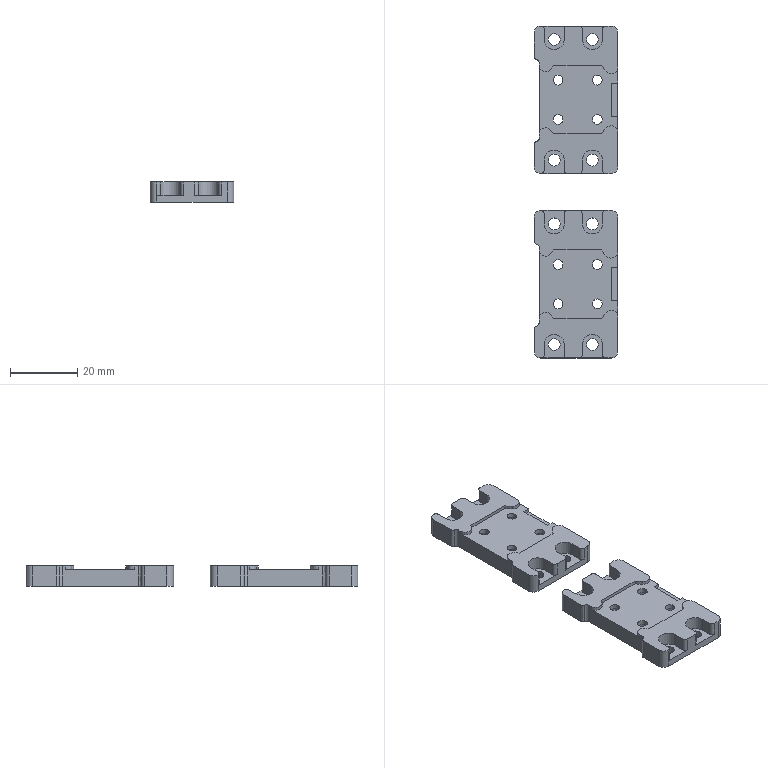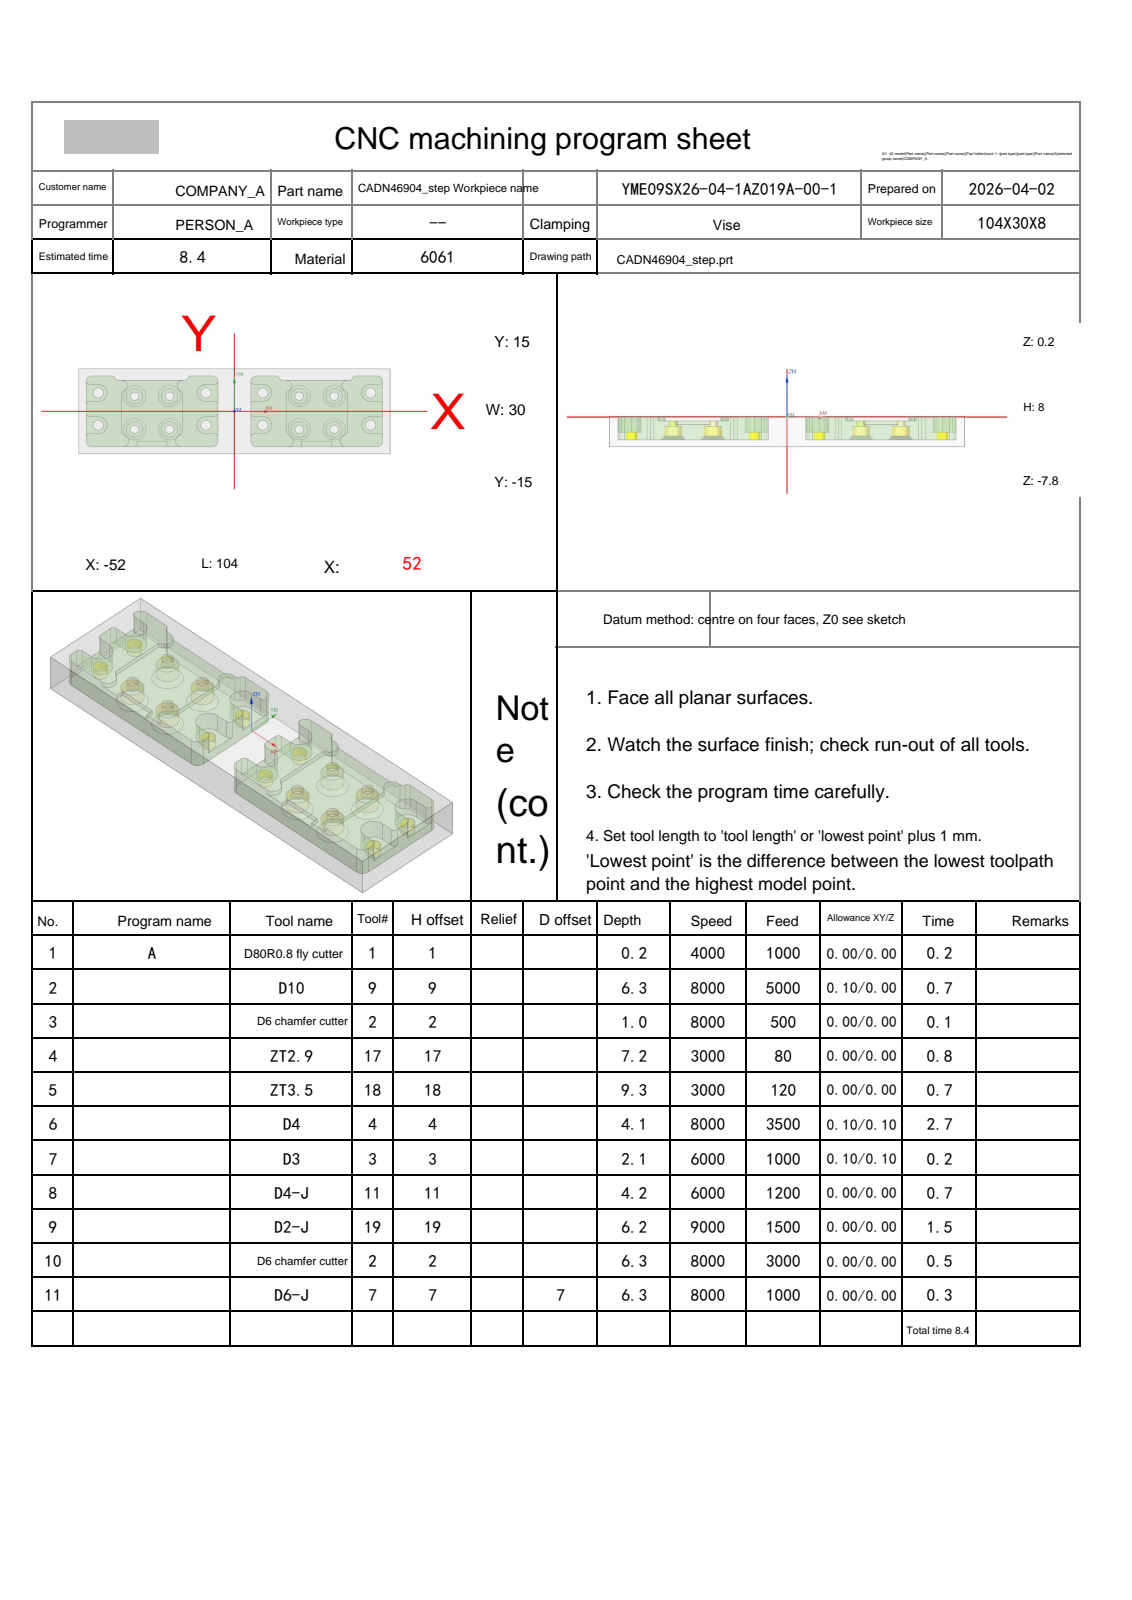NC program | NX | posted by the shop | part box 25 x 99 x 6 mm
Lines 1 to 2900 of 9316, first 1940 of 2898 lines:
%
O0001
(Machine time: 10.55 MIN)
(===Total Tool:10===)
(T1=D80R0.8 fly cutter D=80.  R=0.8  D-  H01 Z=-0.   )
(T9=D10     D=10.  R=0.   D-  H09 Z=-6.1  )
(T2=D6 chamfer cutter   D=6.   R=0.   D-  H02 Z=-6.05 )
(T17=ZT2.9  D=2.9  DR_a=120 D-  H17 Z=-7.   )
(T18=ZT3.5  D=3.5  DR_a=118 D-  H18 Z=-9.05 )
(T4=D4      D=4.   R=0.   D-  H04 Z=-3.9  )
(T3=D3      D=3.   R=0.   D-  H03 Z=-1.9  )
(T11=D4-J   D=4.   R=0.   D11 H11 Z=-4.   )
(T19=D2-J   D=2.   R=0.   D19 H19 Z=-5.95 )
(T7=D6-J    D=6.   R=0.   D7  H07 Z=-6.1  )
G80 G90 G17 G49 G40
G91 G28 Z0
M01
N1 T01 M06
(D80R0.8 fly cutter  D=80. R=0.8 H=01 ce=0.00 di=0.00)
G00 G90 G54 X-94.5 Y0.0 M03 S4000
G43 H01 Z20.
M08
Z2.
G01 Z0.0 F1000.
X-89.5
X89.5
X94.5
Z2.
G00 Z20.
G91 G28 Z0.0
M05
M09
G91 G28 Z0.0
M01
N2 T09 M06
(D10  D=10. R=0. H=09 ce=0.10 di=0.00)
G00 G90 G54 X-27.5 Y-17.6 M03 S8000
G43 H09 Z20.
M08
Z.5
G01 X-47.5 Z.412 F5000.
G02 X-54.6 Y-10.5 Z.363 I0.0 J7.1
G01 Y10.5 Z.271
G02 X-47.5 Y17.6 Z.223 I7.1 J0.0
G01 X-40.936 Z.194
G02 X-36.93 Y16.1 Z.175 I0.0 J-6.1
G01 X-18.57 Z.094
G02 X-14.564 Y17.6 Z.075 I4.006 J-4.6
G01 X-7.5 Z.044
G02 X-.4 Y10.5 Z-.005 I0.0 J-7.1
G01 Y-10.5 Z-.097
G02 X-7.5 Y-17.6 Z-.146 I-7.1 J0.0
G01 X-47.5 Z-.321
G02 X-54.6 Y-10.5 Z-.37 I0.0 J7.1
G01 Y10.5 Z-.462
G02 X-47.5 Y17.6 Z-.511 I7.1 J0.0
G01 X-40.936 Z-.54
G02 X-36.93 Y16.1 Z-.559 I0.0 J-6.1
G01 X-18.57 Z-.639
G02 X-14.564 Y17.6 Z-.658 I4.006 J-4.6
G01 X-7.5 Z-.689
G02 X-.4 Y10.5 Z-.738 I0.0 J-7.1
G01 Y-10.5 Z-.83
G02 X-7.5 Y-17.6 Z-.879 I-7.1 J0.0
G01 X-47.5 Z-1.054
G02 X-54.6 Y-10.5 Z-1.103 I0.0 J7.1
G01 Y10.5 Z-1.195
G02 X-47.5 Y17.6 Z-1.244 I7.1 J0.0
G01 X-40.936 Z-1.273
G02 X-36.93 Y16.1 Z-1.292 I0.0 J-6.1
G01 X-18.57 Z-1.372
G02 X-14.564 Y17.6 Z-1.392 I4.006 J-4.6
G01 X-7.5 Z-1.423
G02 X-.4 Y10.5 Z-1.471 I0.0 J-7.1
G01 Y-10.5 Z-1.563
G02 X-7.5 Y-17.6 Z-1.612 I-7.1 J0.0
G01 X-47.5 Z-1.788
G02 X-54.6 Y-10.5 Z-1.837 I0.0 J7.1
G01 Y10.5 Z-1.929
G02 X-47.5 Y17.6 Z-1.977 I7.1 J0.0
G01 X-40.936 Z-2.006
G02 X-36.93 Y16.1 Z-2.025 I0.0 J-6.1
G01 X-18.57 Z-2.106
G02 X-14.564 Y17.6 Z-2.125 I4.006 J-4.6
G01 X-7.5 Z-2.156
G02 X-.4 Y10.5 Z-2.205 I0.0 J-7.1
G01 Y-10.5 Z-2.297
G02 X-7.5 Y-17.6 Z-2.346 I-7.1 J0.0
G01 X-47.5 Z-2.521
G02 X-54.6 Y-10.5 Z-2.57 I0.0 J7.1
G01 Y10.5 Z-2.662
G02 X-47.5 Y17.6 Z-2.711 I7.1 J0.0
G01 X-40.936 Z-2.74
G02 X-36.93 Y16.1 Z-2.759 I0.0 J-6.1
G01 X-18.57 Z-2.839
G02 X-14.564 Y17.6 Z-2.858 I4.006 J-4.6
G01 X-7.5 Z-2.889
G02 X-.4 Y10.5 Z-2.938 I0.0 J-7.1
G01 Y-10.5 Z-3.03
G02 X-7.5 Y-17.6 Z-3.079 I-7.1 J0.0
G01 X-47.5 Z-3.254
G02 X-54.6 Y-10.5 Z-3.303 I0.0 J7.1
G01 Y10.5 Z-3.395
G02 X-47.5 Y17.6 Z-3.444 I7.1 J0.0
G01 X-40.936 Z-3.473
G02 X-36.93 Y16.1 Z-3.492 I0.0 J-6.1
G01 X-18.57 Z-3.572
G02 X-14.564 Y17.6 Z-3.592 I4.006 J-4.6
G01 X-7.5 Z-3.623
G02 X-.4 Y10.5 Z-3.671 I0.0 J-7.1
G01 Y-10.5 Z-3.763
G02 X-7.5 Y-17.6 Z-3.812 I-7.1 J0.0
G01 X-47.5 Z-3.988
G02 X-54.6 Y-10.5 Z-4.037 I0.0 J7.1
G01 Y10.5 Z-4.129
G02 X-47.5 Y17.6 Z-4.177 I7.1 J0.0
G01 X-40.936 Z-4.206
G02 X-36.93 Y16.1 Z-4.225 I0.0 J-6.1
G01 X-18.57 Z-4.306
G02 X-14.564 Y17.6 Z-4.325 I4.006 J-4.6
G01 X-7.5 Z-4.356
G02 X-.4 Y10.5 Z-4.405 I0.0 J-7.1
G01 Y-10.5 Z-4.497
G02 X-7.5 Y-17.6 Z-4.546 I-7.1 J0.0
G01 X-47.5 Z-4.721
G02 X-54.6 Y-10.5 Z-4.77 I0.0 J7.1
G01 Y10.5 Z-4.862
G02 X-47.5 Y17.6 Z-4.911 I7.1 J0.0
G01 X-40.936 Z-4.94
G02 X-36.93 Y16.1 Z-4.959 I0.0 J-6.1
G01 X-18.57 Z-5.039
G02 X-14.564 Y17.6 Z-5.058 I4.006 J-4.6
G01 X-7.5 Z-5.089
G02 X-.4 Y10.5 Z-5.138 I0.0 J-7.1
G01 Y-10.5 Z-5.23
G02 X-7.5 Y-17.6 Z-5.279 I-7.1 J0.0
G01 X-47.5 Z-5.454
G02 X-54.6 Y-10.5 Z-5.503 I0.0 J7.1
G01 Y10.5 Z-5.595
G02 X-47.5 Y17.6 Z-5.644 I7.1 J0.0
G01 X-40.936 Z-5.673
G02 X-36.93 Y16.1 Z-5.692 I0.0 J-6.1
G01 X-18.57 Z-5.772
G02 X-14.564 Y17.6 Z-5.792 I4.006 J-4.6
G01 X-7.5 Z-5.823
G02 X-.4 Y10.5 Z-5.871 I0.0 J-7.1
G01 Y-10.5 Z-5.963
G02 X-7.5 Y-17.6 Z-6.012 I-7.1 J0.0
G01 X-27.5 Z-6.1
X-47.5
G02 X-54.6 Y-10.5 I0.0 J7.1
G01 Y10.5
G02 X-47.5 Y17.6 I7.1 J0.0
G01 X-40.936
G02 X-36.93 Y16.1 I0.0 J-6.1
G01 X-18.57
G02 X-14.564 Y17.6 I4.006 J-4.6
G01 X-7.5
G02 X-.4 Y10.5 I0.0 J-7.1
G01 Y-10.5
G02 X-7.5 Y-17.6 I-7.1 J0.0
G01 X-27.5
X-28.
Z-5.1
G00 Z20.
X27.5
Z.5
G01 X7.5 Z.412
G02 X.4 Y-10.5 Z.363 I0.0 J7.1
G01 Y10.5 Z.271
G02 X7.5 Y17.6 Z.223 I7.1 J0.0
G01 X14.064 Z.194
G02 X18.07 Y16.1 Z.175 I0.0 J-6.1
G01 X36.43 Z.094
G02 X40.436 Y17.6 Z.075 I4.006 J-4.6
G01 X47.5 Z.044
G02 X54.6 Y10.5 Z-.005 I0.0 J-7.1
G01 Y-10.5 Z-.097
G02 X47.5 Y-17.6 Z-.146 I-7.1 J0.0
G01 X7.5 Z-.321
G02 X.4 Y-10.5 Z-.37 I0.0 J7.1
G01 Y10.5 Z-.462
G02 X7.5 Y17.6 Z-.511 I7.1 J0.0
G01 X14.064 Z-.54
G02 X18.07 Y16.1 Z-.559 I0.0 J-6.1
G01 X36.43 Z-.639
G02 X40.436 Y17.6 Z-.658 I4.006 J-4.6
G01 X47.5 Z-.689
G02 X54.6 Y10.5 Z-.738 I0.0 J-7.1
G01 Y-10.5 Z-.83
G02 X47.5 Y-17.6 Z-.879 I-7.1 J0.0
G01 X7.5 Z-1.054
G02 X.4 Y-10.5 Z-1.103 I0.0 J7.1
G01 Y10.5 Z-1.195
G02 X7.5 Y17.6 Z-1.244 I7.1 J0.0
G01 X14.064 Z-1.273
G02 X18.07 Y16.1 Z-1.292 I0.0 J-6.1
G01 X36.43 Z-1.372
G02 X40.436 Y17.6 Z-1.392 I4.006 J-4.6
G01 X47.5 Z-1.423
G02 X54.6 Y10.5 Z-1.471 I0.0 J-7.1
G01 Y-10.5 Z-1.563
G02 X47.5 Y-17.6 Z-1.612 I-7.1 J0.0
G01 X7.5 Z-1.788
G02 X.4 Y-10.5 Z-1.837 I0.0 J7.1
G01 Y10.5 Z-1.929
G02 X7.5 Y17.6 Z-1.977 I7.1 J0.0
G01 X14.064 Z-2.006
G02 X18.07 Y16.1 Z-2.025 I0.0 J-6.1
G01 X36.43 Z-2.106
G02 X40.436 Y17.6 Z-2.125 I4.006 J-4.6
G01 X47.5 Z-2.156
G02 X54.6 Y10.5 Z-2.205 I0.0 J-7.1
G01 Y-10.5 Z-2.297
G02 X47.5 Y-17.6 Z-2.346 I-7.1 J0.0
G01 X7.5 Z-2.521
G02 X.4 Y-10.5 Z-2.57 I0.0 J7.1
G01 Y10.5 Z-2.662
G02 X7.5 Y17.6 Z-2.711 I7.1 J0.0
G01 X14.064 Z-2.74
G02 X18.07 Y16.1 Z-2.759 I0.0 J-6.1
G01 X36.43 Z-2.839
G02 X40.436 Y17.6 Z-2.858 I4.006 J-4.6
G01 X47.5 Z-2.889
G02 X54.6 Y10.5 Z-2.938 I0.0 J-7.1
G01 Y-10.5 Z-3.03
G02 X47.5 Y-17.6 Z-3.079 I-7.1 J0.0
G01 X7.5 Z-3.254
G02 X.4 Y-10.5 Z-3.303 I0.0 J7.1
G01 Y10.5 Z-3.395
G02 X7.5 Y17.6 Z-3.444 I7.1 J0.0
G01 X14.064 Z-3.473
G02 X18.07 Y16.1 Z-3.492 I0.0 J-6.1
G01 X36.43 Z-3.572
G02 X40.436 Y17.6 Z-3.592 I4.006 J-4.6
G01 X47.5 Z-3.623
G02 X54.6 Y10.5 Z-3.671 I0.0 J-7.1
G01 Y-10.5 Z-3.763
G02 X47.5 Y-17.6 Z-3.812 I-7.1 J0.0
G01 X7.5 Z-3.988
G02 X.4 Y-10.5 Z-4.037 I0.0 J7.1
G01 Y10.5 Z-4.129
G02 X7.5 Y17.6 Z-4.177 I7.1 J0.0
G01 X14.064 Z-4.206
G02 X18.07 Y16.1 Z-4.225 I0.0 J-6.1
G01 X36.43 Z-4.306
G02 X40.436 Y17.6 Z-4.325 I4.006 J-4.6
G01 X47.5 Z-4.356
G02 X54.6 Y10.5 Z-4.405 I0.0 J-7.1
G01 Y-10.5 Z-4.497
G02 X47.5 Y-17.6 Z-4.546 I-7.1 J0.0
G01 X7.5 Z-4.721
G02 X.4 Y-10.5 Z-4.77 I0.0 J7.1
G01 Y10.5 Z-4.862
G02 X7.5 Y17.6 Z-4.911 I7.1 J0.0
G01 X14.064 Z-4.94
G02 X18.07 Y16.1 Z-4.959 I0.0 J-6.1
G01 X36.43 Z-5.039
G02 X40.436 Y17.6 Z-5.058 I4.006 J-4.6
G01 X47.5 Z-5.089
G02 X54.6 Y10.5 Z-5.138 I0.0 J-7.1
G01 Y-10.5 Z-5.23
G02 X47.5 Y-17.6 Z-5.279 I-7.1 J0.0
G01 X7.5 Z-5.454
G02 X.4 Y-10.5 Z-5.503 I0.0 J7.1
G01 Y10.5 Z-5.595
G02 X7.5 Y17.6 Z-5.644 I7.1 J0.0
G01 X14.064 Z-5.673
G02 X18.07 Y16.1 Z-5.692 I0.0 J-6.1
G01 X36.43 Z-5.772
G02 X40.436 Y17.6 Z-5.792 I4.006 J-4.6
G01 X47.5 Z-5.823
G02 X54.6 Y10.5 Z-5.871 I0.0 J-7.1
G01 Y-10.5 Z-5.963
G02 X47.5 Y-17.6 Z-6.012 I-7.1 J0.0
G01 X32.5 Z-6.078
X27.5 Z-6.1
X7.5
G02 X.4 Y-10.5 I0.0 J7.1
G01 Y10.5
G02 X7.5 Y17.6 I7.1 J0.0
G01 X14.064
G02 X18.07 Y16.1 I0.0 J-6.1
G01 X36.43
G02 X40.436 Y17.6 I4.006 J-4.6
G01 X47.5
G02 X54.6 Y10.5 I0.0 J-7.1
G01 Y-10.5
G02 X47.5 Y-17.6 I-7.1 J0.0
G01 X32.5
X27.5
X27.
Z-5.1
G00 Z20.
G91 G28 Z0.0
M05
M09
G91 G28 Z0.0
M01
N3 T02 M06
(D6 chamfer cutter  D=6. R=0. H=02 ce=0.00 di=0.00)
G00 G90 G54 X45.5 Y6.5 M03 S8000
G43 H02 Z20.
M08
G98 G81 X45.5 Y6.5 Z-.8 R1. F500.
Y-4.881
X33.338 Y-6.33
X33.329 Y5.329
X21.662
X21.671 Y-6.338
X9.5 Y-4.881
Y6.5
X-9.5
Y-4.881
X-21.662 Y-6.33
X-21.671 Y5.329
X-33.338
X-33.329 Y-6.338
X-45.5 Y-4.881
Y6.5
G80
G00 Z20.
G91 G28 Z0.0
M05
M09
G91 G28 Z0.0
M01
N4 T17 M06
(ZT2.9 D=2.9 DR_a=120 H=17)
G00 G90 G54 X-33.338 Y5.329 M03 S3000
G43 H17 Z20.
M08
G98 G83 X-33.338 Y5.329 Z-7. R1. F80. Q2.5
X-33.329 Y-6.338
X-21.662 Y-6.33
X-21.671 Y5.329
X21.662
X33.329
X33.338 Y-6.33
X21.671 Y-6.338
G80
G00 Z20.
G91 G28 Z0.0
M05
M09
G91 G28 Z0.0
M01
N5 T18 M06
(ZT3.5 D=3.5 DR_a=118 H=18)
G00 G90 G54 X-45.5 Y-4.881 M03 S3000
G43 H18 Z20.
M08
G98 G83 X-45.5 Y-4.881 Z-9.052 R1. F120. Q3.
Y6.5
X-9.5
Y-4.881
X9.5
Y6.5
X45.5
Y-4.881
G80
G00 Z20.
G91 G28 Z0.0
M05
M09
G91 G28 Z0.0
M01
N6 T04 M06
(D4  D=4. R=0. H=04 ce=0.10 di=0.10)
G00 G90 G54 X-27.5 Y-15.5 M03 S8000
G43 H04 Z20.
M08
Z.275
G01 Z-.225 F3500.
Y-10.9
X-32.1
Y-12.9
X-33.974
G03 X-33.198 Y-10.5 I-3.324 J2.4
X-34.426 Y-7.574 I-4.1 J0.0
X-35.6 Y-6.543 I-9.876 J-10.064
G01 Y5.543
G03 X-35.2 Y5.869 I-8.702 J11.094
X-33.747 Y9. I-2.647 J3.131
X-34.523 Y11.4 I-4.1 J0.0
G01 X-20.477
G03 X-21.253 Y9. I3.324 J-2.4
X-19.8 Y5.869 I4.1 J0.0
X-19.4 Y5.543 I9.102 J10.769
G01 Y-6.543
G03 X-20.574 Y-7.574 I8.702 J-11.094
X-21.802 Y-10.5 I2.872 J-2.926
X-21.026 Y-12.9 I4.1 J0.0
G01 X-22.9
Y-10.9
X-27.5
Y-8.1
X-30.829
G03 X-32.465 Y-5.575 I-6.469 J-2.4
X-32.8 Y-5.255 I-11.837 J-12.062
G01 Y4.295
G03 X-30.958 Y8.6 I-5.047 J4.705
G01 X-24.042
G03 X-22.2 Y4.295 I6.888 J.4
G01 Y-5.255
G03 X-22.535 Y-5.575 I11.502 J-12.382
X-24.171 Y-8.1 I4.833 J-4.925
G01 X-27.5
Y-5.3
X-29.11
G03 X-30. Y-4.11 I-8.188 J-5.2
G01 Y3.298
G03 X-28.69 Y5.8 I-7.847 J5.702
G01 X-26.31
G03 X-25. Y3.298 I9.157 J3.2
G01 Y-4.11
G03 X-25.89 Y-5.3 I7.298 J-6.39
G01 X-27.5
Y-3.5
X-28.174
X-28.2 Y-3.466
Y2.74
G03 X-27.5 Y3.981 I-9.647 J6.26
X-26.8 Y2.74 I10.347 J5.019
G01 Y-3.466
X-26.826 Y-3.5
X-27.5
X-28.
Z.275
G00 Z.5
X-27.5 Y-15.5
Z.05
G01 Z-.45
Y-10.9
X-32.1
Y-12.9
X-33.974
G03 X-33.198 Y-10.5 I-3.324 J2.4
X-34.426 Y-7.574 I-4.1 J0.0
X-35.6 Y-6.543 I-9.876 J-10.064
G01 Y5.543
G03 X-35.2 Y5.869 I-8.702 J11.094
X-33.747 Y9. I-2.647 J3.131
X-34.523 Y11.4 I-4.1 J0.0
G01 X-20.477
G03 X-21.253 Y9. I3.324 J-2.4
X-19.8 Y5.869 I4.1 J0.0
X-19.4 Y5.543 I9.102 J10.769
G01 Y-6.543
G03 X-20.574 Y-7.574 I8.702 J-11.094
X-21.802 Y-10.5 I2.872 J-2.926
X-21.026 Y-12.9 I4.1 J0.0
G01 X-22.9
Y-10.9
X-27.5
Y-8.1
X-30.829
G03 X-32.465 Y-5.575 I-6.469 J-2.4
X-32.8 Y-5.255 I-11.837 J-12.062
G01 Y4.295
G03 X-30.958 Y8.6 I-5.047 J4.705
G01 X-24.042
G03 X-22.2 Y4.295 I6.888 J.4
G01 Y-5.255
G03 X-22.535 Y-5.575 I11.502 J-12.382
X-24.171 Y-8.1 I4.833 J-4.925
G01 X-27.5
Y-5.3
X-29.11
G03 X-30. Y-4.11 I-8.188 J-5.2
G01 Y3.298
G03 X-28.69 Y5.8 I-7.847 J5.702
G01 X-26.31
G03 X-25. Y3.298 I9.157 J3.2
G01 Y-4.11
G03 X-25.89 Y-5.3 I7.298 J-6.39
G01 X-27.5
Y-3.5
X-28.174
X-28.2 Y-3.466
Y2.74
G03 X-27.5 Y3.981 I-9.647 J6.26
X-26.8 Y2.74 I10.347 J5.019
G01 Y-3.466
X-26.826 Y-3.5
X-27.5
X-28.
Z.05
G00 Z.275
X-27.5 Y-15.5
Z-.175
G01 Z-.675
Y-10.9
X-32.1
Y-12.9
X-33.974
G03 X-33.198 Y-10.5 I-3.324 J2.4
X-34.426 Y-7.574 I-4.1 J0.0
X-35.6 Y-6.543 I-9.876 J-10.064
G01 Y5.543
G03 X-35.2 Y5.869 I-8.702 J11.094
X-33.747 Y9. I-2.647 J3.131
X-34.523 Y11.4 I-4.1 J0.0
G01 X-20.477
G03 X-21.253 Y9. I3.324 J-2.4
X-19.8 Y5.869 I4.1 J0.0
X-19.4 Y5.543 I9.102 J10.769
G01 Y-6.543
G03 X-20.574 Y-7.574 I8.702 J-11.094
X-21.802 Y-10.5 I2.872 J-2.926
X-21.026 Y-12.9 I4.1 J0.0
G01 X-22.9
Y-10.9
X-27.5
Y-8.1
X-30.829
G03 X-32.465 Y-5.575 I-6.469 J-2.4
X-32.8 Y-5.255 I-11.837 J-12.062
G01 Y4.295
G03 X-30.958 Y8.6 I-5.047 J4.705
G01 X-24.042
G03 X-22.2 Y4.295 I6.888 J.4
G01 Y-5.255
G03 X-22.535 Y-5.575 I11.502 J-12.382
X-24.171 Y-8.1 I4.833 J-4.925
G01 X-27.5
Y-5.3
X-29.11
G03 X-30. Y-4.11 I-8.188 J-5.2
G01 Y3.298
G03 X-28.69 Y5.8 I-7.847 J5.702
G01 X-26.31
G03 X-25. Y3.298 I9.157 J3.2
G01 Y-4.11
G03 X-25.89 Y-5.3 I7.298 J-6.39
G01 X-27.5
Y-3.5
X-28.174
X-28.2 Y-3.466
Y2.74
G03 X-27.5 Y3.981 I-9.647 J6.26
X-26.8 Y2.74 I10.347 J5.019
G01 Y-3.466
X-26.826 Y-3.5
X-27.5
X-28.
Z-.175
G00 Z.05
X-27.5 Y-15.5
Z-.4
G01 Z-.9
Y-10.9
X-32.1
Y-12.9
X-33.974
G03 X-33.198 Y-10.5 I-3.324 J2.4
X-34.426 Y-7.574 I-4.1 J0.0
X-35.6 Y-6.543 I-9.876 J-10.064
G01 Y5.543
G03 X-35.2 Y5.869 I-8.702 J11.094
X-33.747 Y9. I-2.647 J3.131
X-34.523 Y11.4 I-4.1 J0.0
G01 X-20.477
G03 X-21.253 Y9. I3.324 J-2.4
X-19.8 Y5.869 I4.1 J0.0
X-19.4 Y5.543 I9.102 J10.769
G01 Y-6.543
G03 X-20.574 Y-7.574 I8.702 J-11.094
X-21.802 Y-10.5 I2.872 J-2.926
X-21.026 Y-12.9 I4.1 J0.0
G01 X-22.9
Y-10.9
X-27.5
Y-8.1
X-30.829
G03 X-32.465 Y-5.575 I-6.469 J-2.4
X-32.8 Y-5.255 I-11.837 J-12.062
G01 Y4.295
G03 X-30.958 Y8.6 I-5.047 J4.705
G01 X-24.042
G03 X-22.2 Y4.295 I6.888 J.4
G01 Y-5.255
G03 X-22.535 Y-5.575 I11.502 J-12.382
X-24.171 Y-8.1 I4.833 J-4.925
G01 X-27.5
Y-5.3
X-29.11
G03 X-30. Y-4.11 I-8.188 J-5.2
G01 Y3.298
G03 X-28.69 Y5.8 I-7.847 J5.702
G01 X-26.31
G03 X-25. Y3.298 I9.157 J3.2
G01 Y-4.11
G03 X-25.89 Y-5.3 I7.298 J-6.39
G01 X-27.5
Y-3.5
X-28.174
X-28.2 Y-3.466
Y2.74
G03 X-27.5 Y3.981 I-9.647 J6.26
X-26.8 Y2.74 I10.347 J5.019
G01 Y-3.466
X-26.826 Y-3.5
X-27.5
X-28.
Z-.4
G00 Z20.
X27.5 Y-15.5
Z.275
G01 Z-.225
Y-10.9
X22.9
Y-12.9
X21.026
G03 X21.802 Y-10.5 I-3.324 J2.4
X20.574 Y-7.574 I-4.1 J0.0
X19.4 Y-6.543 I-9.876 J-10.064
G01 Y5.543
G03 X19.8 Y5.869 I-8.702 J11.094
X21.253 Y9. I-2.647 J3.131
X20.477 Y11.4 I-4.1 J0.0
G01 X34.523
G03 X33.747 Y9. I3.324 J-2.4
X35.2 Y5.869 I4.1 J0.0
X35.6 Y5.543 I9.102 J10.769
G01 Y-6.543
G03 X34.426 Y-7.574 I8.702 J-11.094
X33.198 Y-10.5 I2.872 J-2.926
X33.974 Y-12.9 I4.1 J0.0
G01 X32.1
Y-10.9
X27.5
Y-8.1
X24.171
G03 X22.535 Y-5.575 I-6.469 J-2.4
X22.2 Y-5.255 I-11.837 J-12.062
G01 Y4.295
G03 X24.042 Y8.6 I-5.047 J4.705
G01 X30.958
G03 X32.8 Y4.295 I6.888 J.4
G01 Y-5.255
G03 X32.465 Y-5.575 I11.502 J-12.382
X30.829 Y-8.1 I4.833 J-4.925
G01 X27.5
Y-5.3
X25.89
G03 X25. Y-4.11 I-8.188 J-5.2
G01 Y3.298
G03 X26.31 Y5.8 I-7.847 J5.702
G01 X28.69
G03 X30. Y3.298 I9.157 J3.2
G01 Y-4.11
G03 X29.11 Y-5.3 I7.298 J-6.39
G01 X27.5
Y-3.5
X26.826
X26.8 Y-3.466
Y2.74
G03 X27.5 Y3.981 I-9.647 J6.26
X28.2 Y2.74 I10.347 J5.019
G01 Y-3.466
X28.174 Y-3.5
X27.5
X27.
Z.275
G00 Z.5
X27.5 Y-15.5
Z.05
G01 Z-.45
Y-10.9
X22.9
Y-12.9
X21.026
G03 X21.802 Y-10.5 I-3.324 J2.4
X20.574 Y-7.574 I-4.1 J0.0
X19.4 Y-6.543 I-9.876 J-10.064
G01 Y5.543
G03 X19.8 Y5.869 I-8.702 J11.094
X21.253 Y9. I-2.647 J3.131
X20.477 Y11.4 I-4.1 J0.0
G01 X34.523
G03 X33.747 Y9. I3.324 J-2.4
X35.2 Y5.869 I4.1 J0.0
X35.6 Y5.543 I9.102 J10.769
G01 Y-6.543
G03 X34.426 Y-7.574 I8.702 J-11.094
X33.198 Y-10.5 I2.872 J-2.926
X33.974 Y-12.9 I4.1 J0.0
G01 X32.1
Y-10.9
X27.5
Y-8.1
X24.171
G03 X22.535 Y-5.575 I-6.469 J-2.4
X22.2 Y-5.255 I-11.837 J-12.062
G01 Y4.295
G03 X24.042 Y8.6 I-5.047 J4.705
G01 X30.958
G03 X32.8 Y4.295 I6.888 J.4
G01 Y-5.255
G03 X32.465 Y-5.575 I11.502 J-12.382
X30.829 Y-8.1 I4.833 J-4.925
G01 X27.5
Y-5.3
X25.89
G03 X25. Y-4.11 I-8.188 J-5.2
G01 Y3.298
G03 X26.31 Y5.8 I-7.847 J5.702
G01 X28.69
G03 X30. Y3.298 I9.157 J3.2
G01 Y-4.11
G03 X29.11 Y-5.3 I7.298 J-6.39
G01 X27.5
Y-3.5
X26.826
X26.8 Y-3.466
Y2.74
G03 X27.5 Y3.981 I-9.647 J6.26
X28.2 Y2.74 I10.347 J5.019
G01 Y-3.466
X28.174 Y-3.5
X27.5
X27.
Z.05
G00 Z.275
X27.5 Y-15.5
Z-.175
G01 Z-.675
Y-10.9
X22.9
Y-12.9
X21.026
G03 X21.802 Y-10.5 I-3.324 J2.4
X20.574 Y-7.574 I-4.1 J0.0
X19.4 Y-6.543 I-9.876 J-10.064
G01 Y5.543
G03 X19.8 Y5.869 I-8.702 J11.094
X21.253 Y9. I-2.647 J3.131
X20.477 Y11.4 I-4.1 J0.0
G01 X34.523
G03 X33.747 Y9. I3.324 J-2.4
X35.2 Y5.869 I4.1 J0.0
X35.6 Y5.543 I9.102 J10.769
G01 Y-6.543
G03 X34.426 Y-7.574 I8.702 J-11.094
X33.198 Y-10.5 I2.872 J-2.926
X33.974 Y-12.9 I4.1 J0.0
G01 X32.1
Y-10.9
X27.5
Y-8.1
X24.171
G03 X22.535 Y-5.575 I-6.469 J-2.4
X22.2 Y-5.255 I-11.837 J-12.062
G01 Y4.295
G03 X24.042 Y8.6 I-5.047 J4.705
G01 X30.958
G03 X32.8 Y4.295 I6.888 J.4
G01 Y-5.255
G03 X32.465 Y-5.575 I11.502 J-12.382
X30.829 Y-8.1 I4.833 J-4.925
G01 X27.5
Y-5.3
X25.89
G03 X25. Y-4.11 I-8.188 J-5.2
G01 Y3.298
G03 X26.31 Y5.8 I-7.847 J5.702
G01 X28.69
G03 X30. Y3.298 I9.157 J3.2
G01 Y-4.11
G03 X29.11 Y-5.3 I7.298 J-6.39
G01 X27.5
Y-3.5
X26.826
X26.8 Y-3.466
Y2.74
G03 X27.5 Y3.981 I-9.647 J6.26
X28.2 Y2.74 I10.347 J5.019
G01 Y-3.466
X28.174 Y-3.5
X27.5
X27.
Z-.175
G00 Z.05
X27.5 Y-15.5
Z-.4
G01 Z-.9
Y-10.9
X22.9
Y-12.9
X21.026
G03 X21.802 Y-10.5 I-3.324 J2.4
X20.574 Y-7.574 I-4.1 J0.0
X19.4 Y-6.543 I-9.876 J-10.064
G01 Y5.543
G03 X19.8 Y5.869 I-8.702 J11.094
X21.253 Y9. I-2.647 J3.131
X20.477 Y11.4 I-4.1 J0.0
G01 X34.523
G03 X33.747 Y9. I3.324 J-2.4
X35.2 Y5.869 I4.1 J0.0
X35.6 Y5.543 I9.102 J10.769
G01 Y-6.543
G03 X34.426 Y-7.574 I8.702 J-11.094
X33.198 Y-10.5 I2.872 J-2.926
X33.974 Y-12.9 I4.1 J0.0
G01 X32.1
Y-10.9
X27.5
Y-8.1
X24.171
G03 X22.535 Y-5.575 I-6.469 J-2.4
X22.2 Y-5.255 I-11.837 J-12.062
G01 Y4.295
G03 X24.042 Y8.6 I-5.047 J4.705
G01 X30.958
G03 X32.8 Y4.295 I6.888 J.4
G01 Y-5.255
G03 X32.465 Y-5.575 I11.502 J-12.382
X30.829 Y-8.1 I4.833 J-4.925
G01 X27.5
Y-5.3
X25.89
G03 X25. Y-4.11 I-8.188 J-5.2
G01 Y3.298
G03 X26.31 Y5.8 I-7.847 J5.702
G01 X28.69
G03 X30. Y3.298 I9.157 J3.2
G01 Y-4.11
G03 X29.11 Y-5.3 I7.298 J-6.39
G01 X27.5
Y-3.5
X26.826
X26.8 Y-3.466
Y2.74
G03 X27.5 Y3.981 I-9.647 J6.26
X28.2 Y2.74 I10.347 J5.019
G01 Y-3.466
X28.174 Y-3.5
X27.5
X27.
Z-.4
G00 Z20.
G00 G90 X-54.5 Y-4.881 M03 S8000
Z20.
Z.256
G01 Z-.244 F1200.
X-49.9
Y-6.115
G02 X-48.5 Y-5.781 I1.4 J-2.766
G01 X-45.5
G03 X-44.6 Y-4.881 I0.0 J.9
X-45.5 Y-3.981 I-.9 J0.0
G01 X-48.5
G02 X-49.9 Y-3.646 I0.0 J3.1
G01 Y-4.881
Y-5.381
Z.256
G00 Z.5
X-54.5 Y-4.881
Z.013
G01 Z-.488
X-49.9
Y-6.115
G02 X-48.5 Y-5.781 I1.4 J-2.766
G01 X-45.5
G03 X-44.6 Y-4.881 I0.0 J.9
X-45.5 Y-3.981 I-.9 J0.0
G01 X-48.5
G02 X-49.9 Y-3.646 I0.0 J3.1
G01 Y-4.881
Y-5.381
Z.013
G00 Z.256
X-54.5 Y-4.881
Z-.231
G01 Z-.731
X-49.9
Y-6.115
G02 X-48.5 Y-5.781 I1.4 J-2.766
G01 X-45.5
G03 X-44.6 Y-4.881 I0.0 J.9
X-45.5 Y-3.981 I-.9 J0.0
G01 X-48.5
G02 X-49.9 Y-3.646 I0.0 J3.1
G01 Y-4.881
Y-5.381
Z-.231
G00 Z.013
X-54.5 Y-4.881
Z-.475
G01 Z-.975
X-49.9
Y-6.115
G02 X-48.5 Y-5.781 I1.4 J-2.766
G01 X-45.5
G03 X-44.6 Y-4.881 I0.0 J.9
X-45.5 Y-3.981 I-.9 J0.0
G01 X-48.5
G02 X-49.9 Y-3.646 I0.0 J3.1
G01 Y-4.881
Y-5.381
Z-.475
G00 Z-.231
X-54.5 Y-4.881
Z-.719
G01 Z-1.219
X-49.9
Y-6.115
G02 X-48.5 Y-5.781 I1.4 J-2.766
G01 X-45.5
G03 X-44.6 Y-4.881 I0.0 J.9
X-45.5 Y-3.981 I-.9 J0.0
G01 X-48.5
G02 X-49.9 Y-3.646 I0.0 J3.1
G01 Y-4.881
Y-5.381
Z-.719
G00 Z-.475
X-54.5 Y-4.881
Z-.963
G01 Z-1.463
X-49.9
Y-6.115
G02 X-48.5 Y-5.781 I1.4 J-2.766
G01 X-45.5
G03 X-44.6 Y-4.881 I0.0 J.9
X-45.5 Y-3.981 I-.9 J0.0
G01 X-48.5
G02 X-49.9 Y-3.646 I0.0 J3.1
G01 Y-4.881
Y-5.381
Z-.963
G00 Z-.719
X-54.5 Y-4.881
Z-1.206
G01 Z-1.706
X-49.9
Y-6.115
G02 X-48.5 Y-5.781 I1.4 J-2.766
G01 X-45.5
G03 X-44.6 Y-4.881 I0.0 J.9
X-45.5 Y-3.981 I-.9 J0.0
G01 X-48.5
G02 X-49.9 Y-3.646 I0.0 J3.1
G01 Y-4.881
Y-5.381
Z-1.206
G00 Z-.963
X-54.5 Y-4.881
Z-1.45
G01 Z-1.95
X-49.9
Y-6.115
G02 X-48.5 Y-5.781 I1.4 J-2.766
G01 X-45.5
G03 X-44.6 Y-4.881 I0.0 J.9
X-45.5 Y-3.981 I-.9 J0.0
G01 X-48.5
G02 X-49.9 Y-3.646 I0.0 J3.1
G01 Y-4.881
Y-5.381
Z-1.45
G00 Z-1.206
X-54.5 Y-4.881
Z-1.694
G01 Z-2.194
X-49.9
Y-6.115
G02 X-48.5 Y-5.781 I1.4 J-2.766
G01 X-45.5
G03 X-44.6 Y-4.881 I0.0 J.9
X-45.5 Y-3.981 I-.9 J0.0
G01 X-48.5
G02 X-49.9 Y-3.646 I0.0 J3.1
G01 Y-4.881
Y-5.381
Z-1.694
G00 Z-1.45
X-54.5 Y-4.881
Z-1.938
G01 Z-2.438
X-49.9
Y-6.115
G02 X-48.5 Y-5.781 I1.4 J-2.766
G01 X-45.5
G03 X-44.6 Y-4.881 I0.0 J.9
X-45.5 Y-3.981 I-.9 J0.0
G01 X-48.5
G02 X-49.9 Y-3.646 I0.0 J3.1
G01 Y-4.881
Y-5.381
Z-1.938
G00 Z-1.694
X-54.5 Y-4.881
Z-2.181
G01 Z-2.681
X-49.9
Y-6.115
G02 X-48.5 Y-5.781 I1.4 J-2.766
G01 X-45.5
G03 X-44.6 Y-4.881 I0.0 J.9
X-45.5 Y-3.981 I-.9 J0.0
G01 X-48.5
G02 X-49.9 Y-3.646 I0.0 J3.1
G01 Y-4.881
Y-5.381
Z-2.181
G00 Z-1.938
X-54.5 Y-4.881
Z-2.425
G01 Z-2.925
X-49.9
Y-6.115
G02 X-48.5 Y-5.781 I1.4 J-2.766
G01 X-45.5
G03 X-44.6 Y-4.881 I0.0 J.9
X-45.5 Y-3.981 I-.9 J0.0
G01 X-48.5
G02 X-49.9 Y-3.646 I0.0 J3.1
G01 Y-4.881
Y-5.381
Z-2.425
G00 Z-2.181
X-54.5 Y-4.881
Z-2.669
G01 Z-3.169
X-49.9
Y-6.115
G02 X-48.5 Y-5.781 I1.4 J-2.766
G01 X-45.5
G03 X-44.6 Y-4.881 I0.0 J.9
X-45.5 Y-3.981 I-.9 J0.0
G01 X-48.5
G02 X-49.9 Y-3.646 I0.0 J3.1
G01 Y-4.881
Y-5.381
Z-2.669
G00 Z-2.425
X-54.5 Y-4.881
Z-2.913
G01 Z-3.413
X-49.9
Y-6.115
G02 X-48.5 Y-5.781 I1.4 J-2.766
G01 X-45.5
G03 X-44.6 Y-4.881 I0.0 J.9
X-45.5 Y-3.981 I-.9 J0.0
G01 X-48.5
G02 X-49.9 Y-3.646 I0.0 J3.1
G01 Y-4.881
Y-5.381
Z-2.913
G00 Z-2.669
X-54.5 Y-4.881
Z-3.156
G01 Z-3.656
X-49.9
Y-6.115
G02 X-48.5 Y-5.781 I1.4 J-2.766
G01 X-45.5
G03 X-44.6 Y-4.881 I0.0 J.9
X-45.5 Y-3.981 I-.9 J0.0
G01 X-48.5
G02 X-49.9 Y-3.646 I0.0 J3.1
G01 Y-4.881
Y-5.381
Z-3.156
G00 Z-2.913
X-54.5 Y-4.881
Z-3.4
G01 Z-3.9
X-49.9
Y-6.115
G02 X-48.5 Y-5.781 I1.4 J-2.766
G01 X-45.5
G03 X-44.6 Y-4.881 I0.0 J.9
X-45.5 Y-3.981 I-.9 J0.0
G01 X-48.5
G02 X-49.9 Y-3.646 I0.0 J3.1
G01 Y-4.881
Y-5.381
Z-3.4
G00 Z20.
X-54.5 Y6.5
Z.256
G01 Z-.244
X-49.9
Y5.266
G02 X-48.5 Y5.6 I1.4 J-2.766
G01 X-45.5
G03 X-44.6 Y6.5 I0.0 J.9
X-45.5 Y7.4 I-.9 J0.0
G01 X-48.5
G02 X-49.9 Y7.734 I0.0 J3.1
G01 Y6.5
Y6.
Z.256
G00 Z.5
X-54.5 Y6.5
Z.013
G01 Z-.488
X-49.9
Y5.266
G02 X-48.5 Y5.6 I1.4 J-2.766
G01 X-45.5
G03 X-44.6 Y6.5 I0.0 J.9
X-45.5 Y7.4 I-.9 J0.0
G01 X-48.5
G02 X-49.9 Y7.734 I0.0 J3.1
G01 Y6.5
Y6.
Z.013
G00 Z.256
X-54.5 Y6.5
Z-.231
G01 Z-.731
X-49.9
Y5.266
G02 X-48.5 Y5.6 I1.4 J-2.766
G01 X-45.5
G03 X-44.6 Y6.5 I0.0 J.9
X-45.5 Y7.4 I-.9 J0.0
G01 X-48.5
G02 X-49.9 Y7.734 I0.0 J3.1
G01 Y6.5
Y6.
Z-.231
G00 Z.013
X-54.5 Y6.5
Z-.475
G01 Z-.975
X-49.9
Y5.266
G02 X-48.5 Y5.6 I1.4 J-2.766
G01 X-45.5
G03 X-44.6 Y6.5 I0.0 J.9
X-45.5 Y7.4 I-.9 J0.0
G01 X-48.5
G02 X-49.9 Y7.734 I0.0 J3.1
G01 Y6.5
Y6.
Z-.475
G00 Z-.231
X-54.5 Y6.5
Z-.719
G01 Z-1.219
X-49.9
Y5.266
G02 X-48.5 Y5.6 I1.4 J-2.766
G01 X-45.5
G03 X-44.6 Y6.5 I0.0 J.9
X-45.5 Y7.4 I-.9 J0.0
G01 X-48.5
G02 X-49.9 Y7.734 I0.0 J3.1
G01 Y6.5
Y6.
Z-.719
G00 Z-.475
X-54.5 Y6.5
Z-.963
G01 Z-1.463
X-49.9
Y5.266
G02 X-48.5 Y5.6 I1.4 J-2.766
G01 X-45.5
G03 X-44.6 Y6.5 I0.0 J.9
X-45.5 Y7.4 I-.9 J0.0
G01 X-48.5
G02 X-49.9 Y7.734 I0.0 J3.1
G01 Y6.5
Y6.
Z-.963
G00 Z-.719
X-54.5 Y6.5
Z-1.206
G01 Z-1.706
X-49.9
Y5.266
G02 X-48.5 Y5.6 I1.4 J-2.766
G01 X-45.5
G03 X-44.6 Y6.5 I0.0 J.9
X-45.5 Y7.4 I-.9 J0.0
G01 X-48.5
G02 X-49.9 Y7.734 I0.0 J3.1
G01 Y6.5
Y6.
Z-1.206
G00 Z-.963
X-54.5 Y6.5
Z-1.45
G01 Z-1.95
X-49.9
Y5.266
G02 X-48.5 Y5.6 I1.4 J-2.766
G01 X-45.5
G03 X-44.6 Y6.5 I0.0 J.9
X-45.5 Y7.4 I-.9 J0.0
G01 X-48.5
G02 X-49.9 Y7.734 I0.0 J3.1
G01 Y6.5
Y6.
Z-1.45
G00 Z-1.206
X-54.5 Y6.5
Z-1.694
G01 Z-2.194
X-49.9
Y5.266
G02 X-48.5 Y5.6 I1.4 J-2.766
G01 X-45.5
G03 X-44.6 Y6.5 I0.0 J.9
X-45.5 Y7.4 I-.9 J0.0
G01 X-48.5
G02 X-49.9 Y7.734 I0.0 J3.1
G01 Y6.5
Y6.
Z-1.694
G00 Z-1.45
X-54.5 Y6.5
Z-1.938
G01 Z-2.438
X-49.9
Y5.266
G02 X-48.5 Y5.6 I1.4 J-2.766
G01 X-45.5
G03 X-44.6 Y6.5 I0.0 J.9
X-45.5 Y7.4 I-.9 J0.0
G01 X-48.5
G02 X-49.9 Y7.734 I0.0 J3.1
G01 Y6.5
Y6.
Z-1.938
G00 Z-1.694
X-54.5 Y6.5
Z-2.181
G01 Z-2.681
X-49.9
Y5.266
G02 X-48.5 Y5.6 I1.4 J-2.766
G01 X-45.5
G03 X-44.6 Y6.5 I0.0 J.9
X-45.5 Y7.4 I-.9 J0.0
G01 X-48.5
G02 X-49.9 Y7.734 I0.0 J3.1
G01 Y6.5
Y6.
Z-2.181
G00 Z-1.938
X-54.5 Y6.5
Z-2.425
G01 Z-2.925
X-49.9
Y5.266
G02 X-48.5 Y5.6 I1.4 J-2.766
G01 X-45.5
G03 X-44.6 Y6.5 I0.0 J.9
X-45.5 Y7.4 I-.9 J0.0
G01 X-48.5
G02 X-49.9 Y7.734 I0.0 J3.1
G01 Y6.5
Y6.
Z-2.425
G00 Z-2.181
X-54.5 Y6.5
Z-2.669
G01 Z-3.169
X-49.9
Y5.266
G02 X-48.5 Y5.6 I1.4 J-2.766
G01 X-45.5
G03 X-44.6 Y6.5 I0.0 J.9
X-45.5 Y7.4 I-.9 J0.0
G01 X-48.5
G02 X-49.9 Y7.734 I0.0 J3.1
G01 Y6.5
Y6.
Z-2.669
G00 Z-2.425
X-54.5 Y6.5
Z-2.913
G01 Z-3.413
X-49.9
Y5.266
G02 X-48.5 Y5.6 I1.4 J-2.766
G01 X-45.5
G03 X-44.6 Y6.5 I0.0 J.9
X-45.5 Y7.4 I-.9 J0.0
G01 X-48.5
G02 X-49.9 Y7.734 I0.0 J3.1
G01 Y6.5
Y6.
Z-2.913
G00 Z-2.669
X-54.5 Y6.5
Z-3.156
G01 Z-3.656
X-49.9
Y5.266
G02 X-48.5 Y5.6 I1.4 J-2.766
G01 X-45.5
G03 X-44.6 Y6.5 I0.0 J.9
X-45.5 Y7.4 I-.9 J0.0
G01 X-48.5
G02 X-49.9 Y7.734 I0.0 J3.1
G01 Y6.5
Y6.
Z-3.156
G00 Z-2.913
X-54.5 Y6.5
Z-3.4
G01 Z-3.9
X-49.9
Y5.266
G02 X-48.5 Y5.6 I1.4 J-2.766
G01 X-45.5
G03 X-44.6 Y6.5 I0.0 J.9
X-45.5 Y7.4 I-.9 J0.0
G01 X-48.5
G02 X-49.9 Y7.734 I0.0 J3.1
G01 Y6.5
Y6.
Z-3.4
G00 Z20.
X-.5 Y6.5
Z.256
G01 Z-.244
X-5.1
Y7.734
G02 X-6.5 Y7.4 I-1.4 J2.766
G01 X-9.5
G03 X-10.4 Y6.5 I0.0 J-.9
X-9.5 Y5.6 I.9 J0.0
G01 X-6.5
G02 X-5.1 Y5.266 I0.0 J-3.1
G01 Y6.5
Y7.
Z.256
G00 Z.5
X-.5 Y6.5
Z.013
G01 Z-.488
X-5.1
Y7.734
G02 X-6.5 Y7.4 I-1.4 J2.766
G01 X-9.5
G03 X-10.4 Y6.5 I0.0 J-.9
X-9.5 Y5.6 I.9 J0.0
G01 X-6.5
G02 X-5.1 Y5.266 I0.0 J-3.1
G01 Y6.5
Y7.
Z.013
G00 Z.256
X-.5 Y6.5
Z-.231
G01 Z-.731
X-5.1
Y7.734
G02 X-6.5 Y7.4 I-1.4 J2.766
G01 X-9.5
G03 X-10.4 Y6.5 I0.0 J-.9
X-9.5 Y5.6 I.9 J0.0
G01 X-6.5
G02 X-5.1 Y5.266 I0.0 J-3.1
G01 Y6.5
Y7.
Z-.231
G00 Z.013
X-.5 Y6.5
Z-.475
G01 Z-.975
X-5.1
Y7.734
G02 X-6.5 Y7.4 I-1.4 J2.766
G01 X-9.5
G03 X-10.4 Y6.5 I0.0 J-.9
X-9.5 Y5.6 I.9 J0.0
G01 X-6.5
G02 X-5.1 Y5.266 I0.0 J-3.1
G01 Y6.5
Y7.
Z-.475
G00 Z-.231
X-.5 Y6.5
Z-.719
G01 Z-1.219
X-5.1
Y7.734
G02 X-6.5 Y7.4 I-1.4 J2.766
G01 X-9.5
G03 X-10.4 Y6.5 I0.0 J-.9
X-9.5 Y5.6 I.9 J0.0
G01 X-6.5
G02 X-5.1 Y5.266 I0.0 J-3.1
G01 Y6.5
Y7.
Z-.719
G00 Z-.475
X-.5 Y6.5
Z-.963
G01 Z-1.463
X-5.1
Y7.734
G02 X-6.5 Y7.4 I-1.4 J2.766
G01 X-9.5
G03 X-10.4 Y6.5 I0.0 J-.9
X-9.5 Y5.6 I.9 J0.0
G01 X-6.5
G02 X-5.1 Y5.266 I0.0 J-3.1
G01 Y6.5
Y7.
Z-.963
G00 Z-.719
X-.5 Y6.5
Z-1.206
G01 Z-1.706
X-5.1
Y7.734
G02 X-6.5 Y7.4 I-1.4 J2.766
G01 X-9.5
G03 X-10.4 Y6.5 I0.0 J-.9
X-9.5 Y5.6 I.9 J0.0
G01 X-6.5
G02 X-5.1 Y5.266 I0.0 J-3.1
G01 Y6.5
Y7.
Z-1.206
G00 Z-.963
X-.5 Y6.5
Z-1.45
G01 Z-1.95
X-5.1
Y7.734
G02 X-6.5 Y7.4 I-1.4 J2.766
G01 X-9.5
G03 X-10.4 Y6.5 I0.0 J-.9
X-9.5 Y5.6 I.9 J0.0
G01 X-6.5
G02 X-5.1 Y5.266 I0.0 J-3.1
G01 Y6.5
Y7.
Z-1.45
G00 Z-1.206
X-.5 Y6.5
Z-1.694
G01 Z-2.194
X-5.1
Y7.734
G02 X-6.5 Y7.4 I-1.4 J2.766
G01 X-9.5
G03 X-10.4 Y6.5 I0.0 J-.9
X-9.5 Y5.6 I.9 J0.0
G01 X-6.5
G02 X-5.1 Y5.266 I0.0 J-3.1
G01 Y6.5
Y7.
Z-1.694
G00 Z-1.45
X-.5 Y6.5
Z-1.938
G01 Z-2.438
X-5.1
Y7.734
G02 X-6.5 Y7.4 I-1.4 J2.766
G01 X-9.5
G03 X-10.4 Y6.5 I0.0 J-.9
X-9.5 Y5.6 I.9 J0.0
G01 X-6.5
G02 X-5.1 Y5.266 I0.0 J-3.1
G01 Y6.5
Y7.
Z-1.938
G00 Z-1.694
X-.5 Y6.5
Z-2.181
G01 Z-2.681
X-5.1
Y7.734
G02 X-6.5 Y7.4 I-1.4 J2.766
G01 X-9.5
G03 X-10.4 Y6.5 I0.0 J-.9
X-9.5 Y5.6 I.9 J0.0
G01 X-6.5
G02 X-5.1 Y5.266 I0.0 J-3.1
G01 Y6.5
Y7.
Z-2.181
G00 Z-1.938
X-.5 Y6.5
Z-2.425
G01 Z-2.925
X-5.1
Y7.734
G02 X-6.5 Y7.4 I-1.4 J2.766
G01 X-9.5
G03 X-10.4 Y6.5 I0.0 J-.9
X-9.5 Y5.6 I.9 J0.0
G01 X-6.5
G02 X-5.1 Y5.266 I0.0 J-3.1
G01 Y6.5
Y7.
Z-2.425
G00 Z-2.181
X-.5 Y6.5
Z-2.669
G01 Z-3.169
X-5.1
Y7.734
G02 X-6.5 Y7.4 I-1.4 J2.766
G01 X-9.5
G03 X-10.4 Y6.5 I0.0 J-.9
X-9.5 Y5.6 I.9 J0.0
G01 X-6.5
G02 X-5.1 Y5.266 I0.0 J-3.1
G01 Y6.5
Y7.
Z-2.669
G00 Z-2.425
X-.5 Y6.5
Z-2.913
G01 Z-3.413
X-5.1
Y7.734
G02 X-6.5 Y7.4 I-1.4 J2.766
G01 X-9.5
G03 X-10.4 Y6.5 I0.0 J-.9
X-9.5 Y5.6 I.9 J0.0
G01 X-6.5
G02 X-5.1 Y5.266 I0.0 J-3.1
G01 Y6.5
Y7.
Z-2.913
G00 Z-2.669
X-.5 Y6.5
Z-3.156
G01 Z-3.656
X-5.1
Y7.734
G02 X-6.5 Y7.4 I-1.4 J2.766
G01 X-9.5
G03 X-10.4 Y6.5 I0.0 J-.9
X-9.5 Y5.6 I.9 J0.0
G01 X-6.5
G02 X-5.1 Y5.266 I0.0 J-3.1
G01 Y6.5
Y7.
Z-3.156
G00 Z-2.913
X-.5 Y6.5
Z-3.4
G01 Z-3.9
X-5.1
Y7.734
G02 X-6.5 Y7.4 I-1.4 J2.766
G01 X-9.5
G03 X-10.4 Y6.5 I0.0 J-.9
X-9.5 Y5.6 I.9 J0.0
G01 X-6.5
G02 X-5.1 Y5.266 I0.0 J-3.1
G01 Y6.5
Y7.
Z-3.4
G00 Z20.
X-.5 Y-4.881
Z.256
G01 Z-.244
X-5.1
Y-3.646
G02 X-6.5 Y-3.981 I-1.4 J2.766
G01 X-9.5
G03 X-10.4 Y-4.881 I0.0 J-.9
X-9.5 Y-5.781 I.9 J0.0
G01 X-6.5
G02 X-5.1 Y-6.115 I0.0 J-3.1
G01 Y-4.881
Y-4.381
Z.256
G00 Z.5
X-.5 Y-4.881
Z.013
G01 Z-.488
X-5.1
Y-3.646
G02 X-6.5 Y-3.981 I-1.4 J2.766
G01 X-9.5
G03 X-10.4 Y-4.881 I0.0 J-.9
X-9.5 Y-5.781 I.9 J0.0
G01 X-6.5
G02 X-5.1 Y-6.115 I0.0 J-3.1
G01 Y-4.881
Y-4.381
Z.013
G00 Z.256
X-.5 Y-4.881
Z-.231
G01 Z-.731
X-5.1
Y-3.646
G02 X-6.5 Y-3.981 I-1.4 J2.766
G01 X-9.5
G03 X-10.4 Y-4.881 I0.0 J-.9
X-9.5 Y-5.781 I.9 J0.0
G01 X-6.5
G02 X-5.1 Y-6.115 I0.0 J-3.1
G01 Y-4.881
Y-4.381
Z-.231
G00 Z.013
X-.5 Y-4.881
Z-.475
G01 Z-.975
X-5.1
Y-3.646
G02 X-6.5 Y-3.981 I-1.4 J2.766
G01 X-9.5
G03 X-10.4 Y-4.881 I0.0 J-.9
X-9.5 Y-5.781 I.9 J0.0
G01 X-6.5
G02 X-5.1 Y-6.115 I0.0 J-3.1
G01 Y-4.881
Y-4.381
Z-.475
G00 Z-.231
X-.5 Y-4.881
Z-.719
G01 Z-1.219
X-5.1
Y-3.646
G02 X-6.5 Y-3.981 I-1.4 J2.766
G01 X-9.5
G03 X-10.4 Y-4.881 I0.0 J-.9
X-9.5 Y-5.781 I.9 J0.0
G01 X-6.5
G02 X-5.1 Y-6.115 I0.0 J-3.1
G01 Y-4.881
Y-4.381
Z-.719
G00 Z-.475
X-.5 Y-4.881
Z-.963
G01 Z-1.463
X-5.1
Y-3.646
G02 X-6.5 Y-3.981 I-1.4 J2.766
G01 X-9.5
G03 X-10.4 Y-4.881 I0.0 J-.9
X-9.5 Y-5.781 I.9 J0.0
G01 X-6.5
G02 X-5.1 Y-6.115 I0.0 J-3.1
G01 Y-4.881
Y-4.381
Z-.963
G00 Z-.719
X-.5 Y-4.881
Z-1.206
G01 Z-1.706
X-5.1
Y-3.646
G02 X-6.5 Y-3.981 I-1.4 J2.766
G01 X-9.5
G03 X-10.4 Y-4.881 I0.0 J-.9
X-9.5 Y-5.781 I.9 J0.0
G01 X-6.5
G02 X-5.1 Y-6.115 I0.0 J-3.1
G01 Y-4.881
Y-4.381
Z-1.206
G00 Z-.963
X-.5 Y-4.881
Z-1.45
G01 Z-1.95
X-5.1
Y-3.646
G02 X-6.5 Y-3.981 I-1.4 J2.766
G01 X-9.5
G03 X-10.4 Y-4.881 I0.0 J-.9
X-9.5 Y-5.781 I.9 J0.0
G01 X-6.5
G02 X-5.1 Y-6.115 I0.0 J-3.1
G01 Y-4.881
Y-4.381
Z-1.45
G00 Z-1.206
X-.5 Y-4.881
Z-1.694
G01 Z-2.194
X-5.1
Y-3.646
G02 X-6.5 Y-3.981 I-1.4 J2.766
G01 X-9.5
G03 X-10.4 Y-4.881 I0.0 J-.9
X-9.5 Y-5.781 I.9 J0.0
G01 X-6.5
G02 X-5.1 Y-6.115 I0.0 J-3.1
G01 Y-4.881
Y-4.381
Z-1.694
G00 Z-1.45
X-.5 Y-4.881
Z-1.938
G01 Z-2.438
X-5.1
Y-3.646
G02 X-6.5 Y-3.981 I-1.4 J2.766
G01 X-9.5
G03 X-10.4 Y-4.881 I0.0 J-.9
X-9.5 Y-5.781 I.9 J0.0
G01 X-6.5
G02 X-5.1 Y-6.115 I0.0 J-3.1
G01 Y-4.881
Y-4.381
Z-1.938
G00 Z-1.694
X-.5 Y-4.881
Z-2.181
G01 Z-2.681
X-5.1
Y-3.646
G02 X-6.5 Y-3.981 I-1.4 J2.766
G01 X-9.5
G03 X-10.4 Y-4.881 I0.0 J-.9
X-9.5 Y-5.781 I.9 J0.0
G01 X-6.5
G02 X-5.1 Y-6.115 I0.0 J-3.1
G01 Y-4.881
Y-4.381
Z-2.181
G00 Z-1.938
X-.5 Y-4.881
Z-2.425
G01 Z-2.925
X-5.1
Y-3.646
G02 X-6.5 Y-3.981 I-1.4 J2.766
G01 X-9.5
G03 X-10.4 Y-4.881 I0.0 J-.9
X-9.5 Y-5.781 I.9 J0.0
G01 X-6.5
G02 X-5.1 Y-6.115 I0.0 J-3.1
G01 Y-4.881
Y-4.381
Z-2.425
G00 Z-2.181
X-.5 Y-4.881
Z-2.669
G01 Z-3.169
X-5.1
Y-3.646
G02 X-6.5 Y-3.981 I-1.4 J2.766
G01 X-9.5
G03 X-10.4 Y-4.881 I0.0 J-.9
X-9.5 Y-5.781 I.9 J0.0
G01 X-6.5
G02 X-5.1 Y-6.115 I0.0 J-3.1
G01 Y-4.881
Y-4.381
Z-2.669
G00 Z-2.425
X-.5 Y-4.881
Z-2.913
G01 Z-3.413
X-5.1
Y-3.646
G02 X-6.5 Y-3.981 I-1.4 J2.766
G01 X-9.5
G03 X-10.4 Y-4.881 I0.0 J-.9
X-9.5 Y-5.781 I.9 J0.0
G01 X-6.5
G02 X-5.1 Y-6.115 I0.0 J-3.1
G01 Y-4.881
Y-4.381
Z-2.913
G00 Z-2.669
X-.5 Y-4.881
Z-3.156
G01 Z-3.656
X-5.1
Y-3.646
G02 X-6.5 Y-3.981 I-1.4 J2.766
G01 X-9.5
G03 X-10.4 Y-4.881 I0.0 J-.9
X-9.5 Y-5.781 I.9 J0.0
G01 X-6.5
G02 X-5.1 Y-6.115 I0.0 J-3.1
G01 Y-4.881
Y-4.381
Z-3.156
G00 Z-2.913
X-.5 Y-4.881
Z-3.4
G01 Z-3.9
X-5.1
Y-3.646
G02 X-6.5 Y-3.981 I-1.4 J2.766
G01 X-9.5
G03 X-10.4 Y-4.881 I0.0 J-.9
X-9.5 Y-5.781 I.9 J0.0
G01 X-6.5
G02 X-5.1 Y-6.115 I0.0 J-3.1
G01 Y-4.881
Y-4.381
Z-3.4
G00 Z20.
X.5 Y-4.881
Z.256
G01 Z-.244
X5.1
Y-6.115
G02 X6.5 Y-5.781 I1.4 J-2.766
G01 X9.5
G03 X10.4 Y-4.881 I0.0 J.9
X9.5 Y-3.981 I-.9 J0.0
G01 X6.5
G02 X5.1 Y-3.646 I0.0 J3.1
G01 Y-4.881
Y-5.381
Z.256
G00 Z.5
X.5 Y-4.881
Z.013
G01 Z-.488
X5.1
Y-6.115
G02 X6.5 Y-5.781 I1.4 J-2.766
G01 X9.5
G03 X10.4 Y-4.881 I0.0 J.9
X9.5 Y-3.981 I-.9 J0.0
G01 X6.5
G02 X5.1 Y-3.646 I0.0 J3.1
G01 Y-4.881
Y-5.381
Z.013
G00 Z.256
X.5 Y-4.881
Z-.231
G01 Z-.731
X5.1
Y-6.115
G02 X6.5 Y-5.781 I1.4 J-2.766
G01 X9.5
G03 X10.4 Y-4.881 I0.0 J.9
X9.5 Y-3.981 I-.9 J0.0
G01 X6.5
G02 X5.1 Y-3.646 I0.0 J3.1
G01 Y-4.881
Y-5.381
Z-.231
G00 Z.013
X.5 Y-4.881
Z-.475
G01 Z-.975
X5.1
Y-6.115
G02 X6.5 Y-5.781 I1.4 J-2.766
G01 X9.5
G03 X10.4 Y-4.881 I0.0 J.9
X9.5 Y-3.981 I-.9 J0.0
G01 X6.5
G02 X5.1 Y-3.646 I0.0 J3.1
G01 Y-4.881
Y-5.381
Z-.475
G00 Z-.231
X.5 Y-4.881
Z-.719
G01 Z-1.219
X5.1
Y-6.115
G02 X6.5 Y-5.781 I1.4 J-2.766
G01 X9.5
G03 X10.4 Y-4.881 I0.0 J.9
X9.5 Y-3.981 I-.9 J0.0
G01 X6.5
G02 X5.1 Y-3.646 I0.0 J3.1
G01 Y-4.881
Y-5.381
Z-.719
G00 Z-.475
X.5 Y-4.881
Z-.963
G01 Z-1.463
X5.1
Y-6.115
G02 X6.5 Y-5.781 I1.4 J-2.766
G01 X9.5
G03 X10.4 Y-4.881 I0.0 J.9
X9.5 Y-3.981 I-.9 J0.0
G01 X6.5
G02 X5.1 Y-3.646 I0.0 J3.1
G01 Y-4.881
Y-5.381
Z-.963
G00 Z-.719
X.5 Y-4.881
Z-1.206
G01 Z-1.706
X5.1
Y-6.115
G02 X6.5 Y-5.781 I1.4 J-2.766
G01 X9.5
G03 X10.4 Y-4.881 I0.0 J.9
X9.5 Y-3.981 I-.9 J0.0
G01 X6.5
G02 X5.1 Y-3.646 I0.0 J3.1
G01 Y-4.881
Y-5.381
Z-1.206
G00 Z-.963
X.5 Y-4.881
Z-1.45
G01 Z-1.95
X5.1
Y-6.115
G02 X6.5 Y-5.781 I1.4 J-2.766
G01 X9.5
G03 X10.4 Y-4.881 I0.0 J.9
X9.5 Y-3.981 I-.9 J0.0
G01 X6.5
G02 X5.1 Y-3.646 I0.0 J3.1
G01 Y-4.881
Y-5.381
Z-1.45
G00 Z-1.206
X.5 Y-4.881
Z-1.694
G01 Z-2.194
X5.1
Y-6.115
G02 X6.5 Y-5.781 I1.4 J-2.766
G01 X9.5
G03 X10.4 Y-4.881 I0.0 J.9
X9.5 Y-3.981 I-.9 J0.0
G01 X6.5
G02 X5.1 Y-3.646 I0.0 J3.1
G01 Y-4.881
Y-5.381
Z-1.694
G00 Z-1.45
X.5 Y-4.881